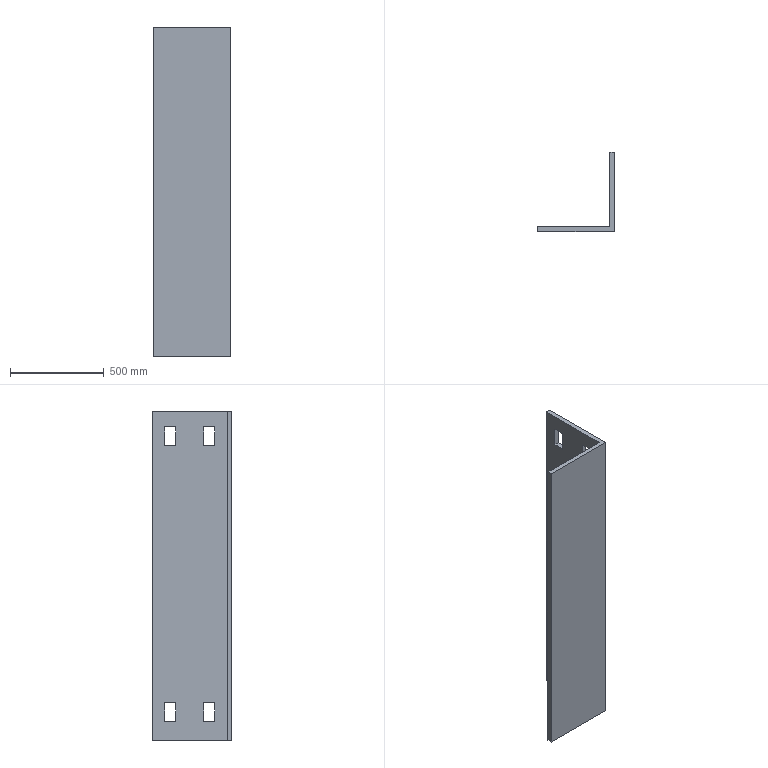Part | SolidWorks | features Extrusion 1, ICE 1 | 1 solid | 24 faces | box 410 x 422.981 x 1750 mm | volume 34749166 mm3 | plane 24
STEP:
#1=CARTESIAN_POINT('',(114.86,92.019,-775.));
#2=VERTEX_POINT('',#1);
#3=CARTESIAN_POINT('',(114.86,152.019,-775.));
#4=VERTEX_POINT('',#3);
#5=CARTESIAN_POINT('',(114.86,152.019,-775.));
#6=DIRECTION('',(0.,1.,0.));
#7=VECTOR('',#6,1000.);
#8=LINE('',#5,#7);
#9=EDGE_CURVE('',#2,#4,#8,.T.);
#10=ORIENTED_EDGE('',*,*,#9,.F.);
#11=CARTESIAN_POINT('',(114.86,92.019,-675.));
#12=VERTEX_POINT('',#11);
#13=CARTESIAN_POINT('',(114.86,92.019,-775.));
#14=DIRECTION('',(0.,0.,-1.));
#15=VECTOR('',#14,1000.);
#16=LINE('',#13,#15);
#17=EDGE_CURVE('',#12,#2,#16,.T.);
#18=ORIENTED_EDGE('',*,*,#17,.F.);
#19=CARTESIAN_POINT('',(114.86,152.019,-675.));
#20=VERTEX_POINT('',#19);
#21=CARTESIAN_POINT('',(114.86,92.019,-675.));
#22=DIRECTION('',(0.,-1.,0.));
#23=VECTOR('',#22,1000.);
#24=LINE('',#21,#23);
#25=EDGE_CURVE('',#20,#12,#24,.T.);
#26=ORIENTED_EDGE('',*,*,#25,.F.);
#27=CARTESIAN_POINT('',(114.86,152.019,-675.));
#28=DIRECTION('',(0.,0.,1.));
#29=VECTOR('',#28,1000.);
#30=LINE('',#27,#29);
#31=EDGE_CURVE('',#4,#20,#30,.T.);
#32=ORIENTED_EDGE('',*,*,#31,.F.);
#33=EDGE_LOOP('',(#10,#18,#26,#32));
#34=FACE_BOUND('',#33,.T.);
#35=CARTESIAN_POINT('',(114.86,360.,-675.));
#36=VERTEX_POINT('',#35);
#37=CARTESIAN_POINT('',(114.86,300.,-675.));
#38=VERTEX_POINT('',#37);
#39=CARTESIAN_POINT('',(114.86,300.,-675.));
#40=DIRECTION('',(0.,-1.,0.));
#41=VECTOR('',#40,1000.);
#42=LINE('',#39,#41);
#43=EDGE_CURVE('',#36,#38,#42,.T.);
#44=ORIENTED_EDGE('',*,*,#43,.F.);
#45=CARTESIAN_POINT('',(114.86,360.,-775.));
#46=VERTEX_POINT('',#45);
#47=CARTESIAN_POINT('',(114.86,360.,-775.));
#48=DIRECTION('',(0.,0.,1.));
#49=VECTOR('',#48,1000.);
#50=LINE('',#47,#49);
#51=EDGE_CURVE('',#46,#36,#50,.T.);
#52=ORIENTED_EDGE('',*,*,#51,.F.);
#53=CARTESIAN_POINT('',(114.86,300.,-775.));
#54=VERTEX_POINT('',#53);
#55=CARTESIAN_POINT('',(114.86,360.,-775.));
#56=DIRECTION('',(0.,1.,0.));
#57=VECTOR('',#56,1000.);
#58=LINE('',#55,#57);
#59=EDGE_CURVE('',#54,#46,#58,.T.);
#60=ORIENTED_EDGE('',*,*,#59,.F.);
#61=CARTESIAN_POINT('',(114.86,300.,-775.));
#62=DIRECTION('',(0.,0.,-1.));
#63=VECTOR('',#62,1000.);
#64=LINE('',#61,#63);
#65=EDGE_CURVE('',#38,#54,#64,.T.);
#66=ORIENTED_EDGE('',*,*,#65,.F.);
#67=EDGE_LOOP('',(#44,#52,#60,#66));
#68=FACE_BOUND('',#67,.T.);
#69=CARTESIAN_POINT('',(114.86,2.019,-875.));
#70=VERTEX_POINT('',#69);
#71=CARTESIAN_POINT('',(114.86,425.,-875.));
#72=VERTEX_POINT('',#71);
#73=CARTESIAN_POINT('',(114.86,2.019,-875.));
#74=DIRECTION('',(0.,1.,0.));
#75=VECTOR('',#74,1000.);
#76=LINE('',#73,#75);
#77=EDGE_CURVE('',#70,#72,#76,.T.);
#78=ORIENTED_EDGE('',*,*,#77,.T.);
#79=CARTESIAN_POINT('',(114.86,425.,875.));
#80=VERTEX_POINT('',#79);
#81=CARTESIAN_POINT('',(114.86,425.,875.));
#82=DIRECTION('',(0.,0.,-1.));
#83=VECTOR('',#82,1000.);
#84=LINE('',#81,#83);
#85=EDGE_CURVE('',#80,#72,#84,.T.);
#86=ORIENTED_EDGE('',*,*,#85,.F.);
#87=CARTESIAN_POINT('',(114.86,2.019,875.));
#88=VERTEX_POINT('',#87);
#89=CARTESIAN_POINT('',(114.86,2.019,875.));
#90=DIRECTION('',(0.,1.,0.));
#91=VECTOR('',#90,1000.);
#92=LINE('',#89,#91);
#93=EDGE_CURVE('',#88,#80,#92,.T.);
#94=ORIENTED_EDGE('',*,*,#93,.F.);
#95=CARTESIAN_POINT('',(114.86,2.019,875.));
#96=DIRECTION('',(0.,0.,-1.));
#97=VECTOR('',#96,1000.);
#98=LINE('',#95,#97);
#99=EDGE_CURVE('',#88,#70,#98,.T.);
#100=ORIENTED_EDGE('',*,*,#99,.T.);
#101=EDGE_LOOP('',(#78,#86,#94,#100));
#102=FACE_OUTER_BOUND('',#101,.T.);
#103=CARTESIAN_POINT('',(114.86,92.019,795.));
#104=VERTEX_POINT('',#103);
#105=CARTESIAN_POINT('',(114.86,92.019,695.));
#106=VERTEX_POINT('',#105);
#107=CARTESIAN_POINT('',(114.86,92.019,695.));
#108=DIRECTION('',(0.,0.,-1.));
#109=VECTOR('',#108,1000.);
#110=LINE('',#107,#109);
#111=EDGE_CURVE('',#104,#106,#110,.T.);
#112=ORIENTED_EDGE('',*,*,#111,.F.);
#113=CARTESIAN_POINT('',(114.86,152.019,795.));
#114=VERTEX_POINT('',#113);
#115=CARTESIAN_POINT('',(114.86,92.019,795.));
#116=DIRECTION('',(0.,-1.,0.));
#117=VECTOR('',#116,1000.);
#118=LINE('',#115,#117);
#119=EDGE_CURVE('',#114,#104,#118,.T.);
#120=ORIENTED_EDGE('',*,*,#119,.F.);
#121=CARTESIAN_POINT('',(114.86,152.019,695.));
#122=VERTEX_POINT('',#121);
#123=CARTESIAN_POINT('',(114.86,152.019,795.));
#124=DIRECTION('',(0.,0.,1.));
#125=VECTOR('',#124,1000.);
#126=LINE('',#123,#125);
#127=EDGE_CURVE('',#122,#114,#126,.T.);
#128=ORIENTED_EDGE('',*,*,#127,.F.);
#129=CARTESIAN_POINT('',(114.86,152.019,695.));
#130=DIRECTION('',(0.,1.,0.));
#131=VECTOR('',#130,1000.);
#132=LINE('',#129,#131);
#133=EDGE_CURVE('',#106,#122,#132,.T.);
#134=ORIENTED_EDGE('',*,*,#133,.F.);
#135=EDGE_LOOP('',(#112,#120,#128,#134));
#136=FACE_BOUND('',#135,.T.);
#137=CARTESIAN_POINT('',(114.86,360.,695.));
#138=VERTEX_POINT('',#137);
#139=CARTESIAN_POINT('',(114.86,360.,795.));
#140=VERTEX_POINT('',#139);
#141=CARTESIAN_POINT('',(114.86,360.,795.));
#142=DIRECTION('',(0.,0.,1.));
#143=VECTOR('',#142,1000.);
#144=LINE('',#141,#143);
#145=EDGE_CURVE('',#138,#140,#144,.T.);
#146=ORIENTED_EDGE('',*,*,#145,.F.);
#147=CARTESIAN_POINT('',(114.86,300.,695.));
#148=VERTEX_POINT('',#147);
#149=CARTESIAN_POINT('',(114.86,360.,695.));
#150=DIRECTION('',(0.,1.,0.));
#151=VECTOR('',#150,1000.);
#152=LINE('',#149,#151);
#153=EDGE_CURVE('',#148,#138,#152,.T.);
#154=ORIENTED_EDGE('',*,*,#153,.F.);
#155=CARTESIAN_POINT('',(114.86,300.,795.));
#156=VERTEX_POINT('',#155);
#157=CARTESIAN_POINT('',(114.86,300.,795.));
#158=DIRECTION('',(0.,0.,-1.));
#159=VECTOR('',#158,1000.);
#160=LINE('',#157,#159);
#161=EDGE_CURVE('',#156,#148,#160,.T.);
#162=ORIENTED_EDGE('',*,*,#161,.F.);
#163=CARTESIAN_POINT('',(114.86,300.,795.));
#164=DIRECTION('',(0.,-1.,0.));
#165=VECTOR('',#164,1000.);
#166=LINE('',#163,#165);
#167=EDGE_CURVE('',#140,#156,#166,.T.);
#168=ORIENTED_EDGE('',*,*,#167,.F.);
#169=EDGE_LOOP('',(#146,#154,#162,#168));
#170=FACE_BOUND('',#169,.T.);
#171=CARTESIAN_POINT('',(114.86,2.019,875.));
#172=DIRECTION('',(-1.,0.,0.));
#173=DIRECTION('',(0.,0.,1.));
#174=AXIS2_PLACEMENT_3D('',#171,#172,#173);
#175=PLANE('',#174);
#176=ADVANCED_FACE('',(#34,#68,#102,#136,#170),#175,.F.);
#177=CARTESIAN_POINT('',(89.86,152.019,-775.));
#178=VERTEX_POINT('',#177);
#179=CARTESIAN_POINT('',(89.86,92.019,-775.));
#180=VERTEX_POINT('',#179);
#181=CARTESIAN_POINT('',(89.86,425.,-775.));
#182=DIRECTION('',(0.,-1.,0.));
#183=VECTOR('',#182,1000.);
#184=LINE('',#181,#183);
#185=EDGE_CURVE('',#178,#180,#184,.T.);
#186=ORIENTED_EDGE('',*,*,#185,.F.);
#187=CARTESIAN_POINT('',(89.86,152.019,-675.));
#188=VERTEX_POINT('',#187);
#189=CARTESIAN_POINT('',(89.86,152.019,875.));
#190=DIRECTION('',(0.,0.,-1.));
#191=VECTOR('',#190,1000.);
#192=LINE('',#189,#191);
#193=EDGE_CURVE('',#188,#178,#192,.T.);
#194=ORIENTED_EDGE('',*,*,#193,.F.);
#195=CARTESIAN_POINT('',(89.86,92.019,-675.));
#196=VERTEX_POINT('',#195);
#197=CARTESIAN_POINT('',(89.86,425.,-675.));
#198=DIRECTION('',(0.,1.,0.));
#199=VECTOR('',#198,1000.);
#200=LINE('',#197,#199);
#201=EDGE_CURVE('',#196,#188,#200,.T.);
#202=ORIENTED_EDGE('',*,*,#201,.F.);
#203=CARTESIAN_POINT('',(89.86,92.019,875.));
#204=DIRECTION('',(0.,0.,1.));
#205=VECTOR('',#204,1000.);
#206=LINE('',#203,#205);
#207=EDGE_CURVE('',#180,#196,#206,.T.);
#208=ORIENTED_EDGE('',*,*,#207,.F.);
#209=EDGE_LOOP('',(#186,#194,#202,#208));
#210=FACE_BOUND('',#209,.T.);
#211=CARTESIAN_POINT('',(89.86,300.,-675.));
#212=VERTEX_POINT('',#211);
#213=CARTESIAN_POINT('',(89.86,360.,-675.));
#214=VERTEX_POINT('',#213);
#215=CARTESIAN_POINT('',(89.86,425.,-675.));
#216=DIRECTION('',(0.,1.,0.));
#217=VECTOR('',#216,1000.);
#218=LINE('',#215,#217);
#219=EDGE_CURVE('',#212,#214,#218,.T.);
#220=ORIENTED_EDGE('',*,*,#219,.F.);
#221=CARTESIAN_POINT('',(89.86,300.,-775.));
#222=VERTEX_POINT('',#221);
#223=CARTESIAN_POINT('',(89.86,300.,875.));
#224=DIRECTION('',(0.,0.,1.));
#225=VECTOR('',#224,1000.);
#226=LINE('',#223,#225);
#227=EDGE_CURVE('',#222,#212,#226,.T.);
#228=ORIENTED_EDGE('',*,*,#227,.F.);
#229=CARTESIAN_POINT('',(89.86,360.,-775.));
#230=VERTEX_POINT('',#229);
#231=CARTESIAN_POINT('',(89.86,425.,-775.));
#232=DIRECTION('',(0.,-1.,0.));
#233=VECTOR('',#232,1000.);
#234=LINE('',#231,#233);
#235=EDGE_CURVE('',#230,#222,#234,.T.);
#236=ORIENTED_EDGE('',*,*,#235,.F.);
#237=CARTESIAN_POINT('',(89.86,360.,875.));
#238=DIRECTION('',(0.,0.,-1.));
#239=VECTOR('',#238,1000.);
#240=LINE('',#237,#239);
#241=EDGE_CURVE('',#214,#230,#240,.T.);
#242=ORIENTED_EDGE('',*,*,#241,.F.);
#243=EDGE_LOOP('',(#220,#228,#236,#242));
#244=FACE_BOUND('',#243,.T.);
#245=CARTESIAN_POINT('',(89.86,425.,-875.));
#246=VERTEX_POINT('',#245);
#247=CARTESIAN_POINT('',(89.86,27.019,-875.));
#248=VERTEX_POINT('',#247);
#249=CARTESIAN_POINT('',(89.86,425.,-875.));
#250=DIRECTION('',(0.,-1.,0.));
#251=VECTOR('',#250,1000.);
#252=LINE('',#249,#251);
#253=EDGE_CURVE('',#246,#248,#252,.T.);
#254=ORIENTED_EDGE('',*,*,#253,.T.);
#255=CARTESIAN_POINT('',(89.86,27.019,875.));
#256=VERTEX_POINT('',#255);
#257=CARTESIAN_POINT('',(89.86,27.019,875.));
#258=DIRECTION('',(0.,0.,-1.));
#259=VECTOR('',#258,1000.);
#260=LINE('',#257,#259);
#261=EDGE_CURVE('',#256,#248,#260,.T.);
#262=ORIENTED_EDGE('',*,*,#261,.F.);
#263=CARTESIAN_POINT('',(89.86,425.,875.));
#264=VERTEX_POINT('',#263);
#265=CARTESIAN_POINT('',(89.86,425.,875.));
#266=DIRECTION('',(0.,-1.,0.));
#267=VECTOR('',#266,1000.);
#268=LINE('',#265,#267);
#269=EDGE_CURVE('',#264,#256,#268,.T.);
#270=ORIENTED_EDGE('',*,*,#269,.F.);
#271=CARTESIAN_POINT('',(89.86,425.,875.));
#272=DIRECTION('',(0.,0.,-1.));
#273=VECTOR('',#272,1000.);
#274=LINE('',#271,#273);
#275=EDGE_CURVE('',#264,#246,#274,.T.);
#276=ORIENTED_EDGE('',*,*,#275,.T.);
#277=EDGE_LOOP('',(#254,#262,#270,#276));
#278=FACE_OUTER_BOUND('',#277,.T.);
#279=CARTESIAN_POINT('',(89.86,92.019,695.));
#280=VERTEX_POINT('',#279);
#281=CARTESIAN_POINT('',(89.86,92.019,795.));
#282=VERTEX_POINT('',#281);
#283=CARTESIAN_POINT('',(89.86,92.019,875.));
#284=DIRECTION('',(0.,0.,1.));
#285=VECTOR('',#284,1000.);
#286=LINE('',#283,#285);
#287=EDGE_CURVE('',#280,#282,#286,.T.);
#288=ORIENTED_EDGE('',*,*,#287,.F.);
#289=CARTESIAN_POINT('',(89.86,152.019,695.));
#290=VERTEX_POINT('',#289);
#291=CARTESIAN_POINT('',(89.86,425.,695.));
#292=DIRECTION('',(0.,-1.,0.));
#293=VECTOR('',#292,1000.);
#294=LINE('',#291,#293);
#295=EDGE_CURVE('',#290,#280,#294,.T.);
#296=ORIENTED_EDGE('',*,*,#295,.F.);
#297=CARTESIAN_POINT('',(89.86,152.019,795.));
#298=VERTEX_POINT('',#297);
#299=CARTESIAN_POINT('',(89.86,152.019,875.));
#300=DIRECTION('',(0.,0.,-1.));
#301=VECTOR('',#300,1000.);
#302=LINE('',#299,#301);
#303=EDGE_CURVE('',#298,#290,#302,.T.);
#304=ORIENTED_EDGE('',*,*,#303,.F.);
#305=CARTESIAN_POINT('',(89.86,425.,795.));
#306=DIRECTION('',(0.,1.,0.));
#307=VECTOR('',#306,1000.);
#308=LINE('',#305,#307);
#309=EDGE_CURVE('',#282,#298,#308,.T.);
#310=ORIENTED_EDGE('',*,*,#309,.F.);
#311=EDGE_LOOP('',(#288,#296,#304,#310));
#312=FACE_BOUND('',#311,.T.);
#313=CARTESIAN_POINT('',(89.86,360.,795.));
#314=VERTEX_POINT('',#313);
#315=CARTESIAN_POINT('',(89.86,360.,695.));
#316=VERTEX_POINT('',#315);
#317=CARTESIAN_POINT('',(89.86,360.,875.));
#318=DIRECTION('',(0.,0.,-1.));
#319=VECTOR('',#318,1000.);
#320=LINE('',#317,#319);
#321=EDGE_CURVE('',#314,#316,#320,.T.);
#322=ORIENTED_EDGE('',*,*,#321,.F.);
#323=CARTESIAN_POINT('',(89.86,300.,795.));
#324=VERTEX_POINT('',#323);
#325=CARTESIAN_POINT('',(89.86,425.,795.));
#326=DIRECTION('',(0.,1.,0.));
#327=VECTOR('',#326,1000.);
#328=LINE('',#325,#327);
#329=EDGE_CURVE('',#324,#314,#328,.T.);
#330=ORIENTED_EDGE('',*,*,#329,.F.);
#331=CARTESIAN_POINT('',(89.86,300.,695.));
#332=VERTEX_POINT('',#331);
#333=CARTESIAN_POINT('',(89.86,300.,875.));
#334=DIRECTION('',(0.,0.,1.));
#335=VECTOR('',#334,1000.);
#336=LINE('',#333,#335);
#337=EDGE_CURVE('',#332,#324,#336,.T.);
#338=ORIENTED_EDGE('',*,*,#337,.F.);
#339=CARTESIAN_POINT('',(89.86,425.,695.));
#340=DIRECTION('',(0.,-1.,0.));
#341=VECTOR('',#340,1000.);
#342=LINE('',#339,#341);
#343=EDGE_CURVE('',#316,#332,#342,.T.);
#344=ORIENTED_EDGE('',*,*,#343,.F.);
#345=EDGE_LOOP('',(#322,#330,#338,#344));
#346=FACE_BOUND('',#345,.T.);
#347=CARTESIAN_POINT('',(89.86,425.,875.));
#348=DIRECTION('',(1.,0.,0.));
#349=DIRECTION('',(0.,0.,-1.));
#350=AXIS2_PLACEMENT_3D('',#347,#348,#349);
#351=PLANE('',#350);
#352=ADVANCED_FACE('',(#210,#244,#278,#312,#346),#351,.F.);
#353=CARTESIAN_POINT('',(-295.14,2.019,-875.));
#354=VERTEX_POINT('',#353);
#355=CARTESIAN_POINT('',(-295.14,2.019,-875.));
#356=DIRECTION('',(1.,0.,0.));
#357=VECTOR('',#356,1000.);
#358=LINE('',#355,#357);
#359=EDGE_CURVE('',#354,#70,#358,.T.);
#360=ORIENTED_EDGE('',*,*,#359,.T.);
#361=ORIENTED_EDGE('',*,*,#99,.F.);
#362=CARTESIAN_POINT('',(-295.14,2.019,875.));
#363=VERTEX_POINT('',#362);
#364=CARTESIAN_POINT('',(-295.14,2.019,875.));
#365=DIRECTION('',(1.,0.,0.));
#366=VECTOR('',#365,1000.);
#367=LINE('',#364,#366);
#368=EDGE_CURVE('',#363,#88,#367,.T.);
#369=ORIENTED_EDGE('',*,*,#368,.F.);
#370=CARTESIAN_POINT('',(-295.14,2.019,875.));
#371=DIRECTION('',(0.,0.,-1.));
#372=VECTOR('',#371,1000.);
#373=LINE('',#370,#372);
#374=EDGE_CURVE('',#363,#354,#373,.T.);
#375=ORIENTED_EDGE('',*,*,#374,.T.);
#376=EDGE_LOOP('',(#360,#361,#369,#375));
#377=FACE_OUTER_BOUND('',#376,.T.);
#378=CARTESIAN_POINT('',(-295.14,2.019,875.));
#379=DIRECTION('',(0.,1.,0.));
#380=DIRECTION('',(0.,0.,1.));
#381=AXIS2_PLACEMENT_3D('',#378,#379,#380);
#382=PLANE('',#381);
#383=ADVANCED_FACE('',(#377),#382,.F.);
#384=CARTESIAN_POINT('',(114.86,425.,-875.));
#385=DIRECTION('',(-1.,0.,0.));
#386=VECTOR('',#385,1000.);
#387=LINE('',#384,#386);
#388=EDGE_CURVE('',#72,#246,#387,.T.);
#389=ORIENTED_EDGE('',*,*,#388,.T.);
#390=ORIENTED_EDGE('',*,*,#275,.F.);
#391=CARTESIAN_POINT('',(114.86,425.,875.));
#392=DIRECTION('',(-1.,0.,0.));
#393=VECTOR('',#392,1000.);
#394=LINE('',#391,#393);
#395=EDGE_CURVE('',#80,#264,#394,.T.);
#396=ORIENTED_EDGE('',*,*,#395,.F.);
#397=ORIENTED_EDGE('',*,*,#85,.T.);
#398=EDGE_LOOP('',(#389,#390,#396,#397));
#399=FACE_OUTER_BOUND('',#398,.T.);
#400=CARTESIAN_POINT('',(114.86,425.,875.));
#401=DIRECTION('',(0.,-1.,0.));
#402=DIRECTION('',(0.,0.,-1.));
#403=AXIS2_PLACEMENT_3D('',#400,#401,#402);
#404=PLANE('',#403);
#405=ADVANCED_FACE('',(#399),#404,.F.);
#406=CARTESIAN_POINT('',(-295.14,27.019,-875.));
#407=VERTEX_POINT('',#406);
#408=CARTESIAN_POINT('',(89.86,27.019,-875.));
#409=DIRECTION('',(-1.,0.,0.));
#410=VECTOR('',#409,1000.);
#411=LINE('',#408,#410);
#412=EDGE_CURVE('',#248,#407,#411,.T.);
#413=ORIENTED_EDGE('',*,*,#412,.T.);
#414=CARTESIAN_POINT('',(-295.14,27.019,875.));
#415=VERTEX_POINT('',#414);
#416=CARTESIAN_POINT('',(-295.14,27.019,875.));
#417=DIRECTION('',(0.,0.,-1.));
#418=VECTOR('',#417,1000.);
#419=LINE('',#416,#418);
#420=EDGE_CURVE('',#415,#407,#419,.T.);
#421=ORIENTED_EDGE('',*,*,#420,.F.);
#422=CARTESIAN_POINT('',(89.86,27.019,875.));
#423=DIRECTION('',(-1.,0.,0.));
#424=VECTOR('',#423,1000.);
#425=LINE('',#422,#424);
#426=EDGE_CURVE('',#256,#415,#425,.T.);
#427=ORIENTED_EDGE('',*,*,#426,.F.);
#428=ORIENTED_EDGE('',*,*,#261,.T.);
#429=EDGE_LOOP('',(#413,#421,#427,#428));
#430=FACE_OUTER_BOUND('',#429,.T.);
#431=CARTESIAN_POINT('',(89.86,27.019,875.));
#432=DIRECTION('',(0.,-1.,0.));
#433=DIRECTION('',(1.,0.,0.));
#434=AXIS2_PLACEMENT_3D('',#431,#432,#433);
#435=PLANE('',#434);
#436=ADVANCED_FACE('',(#430),#435,.F.);
#437=CARTESIAN_POINT('',(-295.14,27.019,-875.));
#438=DIRECTION('',(0.,-1.,0.));
#439=VECTOR('',#438,1000.);
#440=LINE('',#437,#439);
#441=EDGE_CURVE('',#407,#354,#440,.T.);
#442=ORIENTED_EDGE('',*,*,#441,.T.);
#443=ORIENTED_EDGE('',*,*,#374,.F.);
#444=CARTESIAN_POINT('',(-295.14,27.019,875.));
#445=DIRECTION('',(0.,-1.,0.));
#446=VECTOR('',#445,1000.);
#447=LINE('',#444,#446);
#448=EDGE_CURVE('',#415,#363,#447,.T.);
#449=ORIENTED_EDGE('',*,*,#448,.F.);
#450=ORIENTED_EDGE('',*,*,#420,.T.);
#451=EDGE_LOOP('',(#442,#443,#449,#450));
#452=FACE_OUTER_BOUND('',#451,.T.);
#453=CARTESIAN_POINT('',(-295.14,27.019,875.));
#454=DIRECTION('',(1.,0.,0.));
#455=DIRECTION('',(0.,0.,-1.));
#456=AXIS2_PLACEMENT_3D('',#453,#454,#455);
#457=PLANE('',#456);
#458=ADVANCED_FACE('',(#452),#457,.F.);
#459=ORIENTED_EDGE('',*,*,#368,.T.);
#460=ORIENTED_EDGE('',*,*,#93,.T.);
#461=ORIENTED_EDGE('',*,*,#395,.T.);
#462=ORIENTED_EDGE('',*,*,#269,.T.);
#463=ORIENTED_EDGE('',*,*,#426,.T.);
#464=ORIENTED_EDGE('',*,*,#448,.T.);
#465=EDGE_LOOP('',(#459,#460,#461,#462,#463,#464));
#466=FACE_OUTER_BOUND('',#465,.T.);
#467=CARTESIAN_POINT('',(0.,0.,875.));
#468=DIRECTION('',(0.,0.,1.));
#469=DIRECTION('',(1.,0.,0.));
#470=AXIS2_PLACEMENT_3D('',#467,#468,#469);
#471=PLANE('',#470);
#472=ADVANCED_FACE('',(#466),#471,.T.);
#473=ORIENTED_EDGE('',*,*,#359,.F.);
#474=ORIENTED_EDGE('',*,*,#441,.F.);
#475=ORIENTED_EDGE('',*,*,#412,.F.);
#476=ORIENTED_EDGE('',*,*,#253,.F.);
#477=ORIENTED_EDGE('',*,*,#388,.F.);
#478=ORIENTED_EDGE('',*,*,#77,.F.);
#479=EDGE_LOOP('',(#473,#474,#475,#476,#477,#478));
#480=FACE_OUTER_BOUND('',#479,.T.);
#481=CARTESIAN_POINT('',(0.,0.,-875.));
#482=DIRECTION('',(0.,0.,1.));
#483=DIRECTION('',(1.,0.,0.));
#484=AXIS2_PLACEMENT_3D('',#481,#482,#483);
#485=PLANE('',#484);
#486=ADVANCED_FACE('',(#480),#485,.F.);
#487=ORIENTED_EDGE('',*,*,#219,.T.);
#488=CARTESIAN_POINT('',(114.86,360.,-675.));
#489=DIRECTION('',(-1.,0.,0.));
#490=VECTOR('',#489,1000.);
#491=LINE('',#488,#490);
#492=EDGE_CURVE('',#36,#214,#491,.T.);
#493=ORIENTED_EDGE('',*,*,#492,.F.);
#494=ORIENTED_EDGE('',*,*,#43,.T.);
#495=CARTESIAN_POINT('',(114.86,300.,-675.));
#496=DIRECTION('',(-1.,0.,0.));
#497=VECTOR('',#496,1000.);
#498=LINE('',#495,#497);
#499=EDGE_CURVE('',#38,#212,#498,.T.);
#500=ORIENTED_EDGE('',*,*,#499,.T.);
#501=EDGE_LOOP('',(#487,#493,#494,#500));
#502=FACE_OUTER_BOUND('',#501,.T.);
#503=CARTESIAN_POINT('',(114.86,300.,-675.));
#504=DIRECTION('',(0.,0.,-1.));
#505=DIRECTION('',(-1.,0.,0.));
#506=AXIS2_PLACEMENT_3D('',#503,#504,#505);
#507=PLANE('',#506);
#508=ADVANCED_FACE('',(#502),#507,.T.);
#509=ORIENTED_EDGE('',*,*,#227,.T.);
#510=ORIENTED_EDGE('',*,*,#499,.F.);
#511=ORIENTED_EDGE('',*,*,#65,.T.);
#512=CARTESIAN_POINT('',(114.86,300.,-775.));
#513=DIRECTION('',(-1.,0.,0.));
#514=VECTOR('',#513,1000.);
#515=LINE('',#512,#514);
#516=EDGE_CURVE('',#54,#222,#515,.T.);
#517=ORIENTED_EDGE('',*,*,#516,.T.);
#518=EDGE_LOOP('',(#509,#510,#511,#517));
#519=FACE_OUTER_BOUND('',#518,.T.);
#520=CARTESIAN_POINT('',(114.86,300.,-775.));
#521=DIRECTION('',(0.,1.,0.));
#522=DIRECTION('',(0.,0.,1.));
#523=AXIS2_PLACEMENT_3D('',#520,#521,#522);
#524=PLANE('',#523);
#525=ADVANCED_FACE('',(#519),#524,.T.);
#526=ORIENTED_EDGE('',*,*,#235,.T.);
#527=ORIENTED_EDGE('',*,*,#516,.F.);
#528=ORIENTED_EDGE('',*,*,#59,.T.);
#529=CARTESIAN_POINT('',(114.86,360.,-775.));
#530=DIRECTION('',(-1.,0.,0.));
#531=VECTOR('',#530,1000.);
#532=LINE('',#529,#531);
#533=EDGE_CURVE('',#46,#230,#532,.T.);
#534=ORIENTED_EDGE('',*,*,#533,.T.);
#535=EDGE_LOOP('',(#526,#527,#528,#534));
#536=FACE_OUTER_BOUND('',#535,.T.);
#537=CARTESIAN_POINT('',(114.86,360.,-775.));
#538=DIRECTION('',(0.,0.,1.));
#539=DIRECTION('',(1.,0.,0.));
#540=AXIS2_PLACEMENT_3D('',#537,#538,#539);
#541=PLANE('',#540);
#542=ADVANCED_FACE('',(#536),#541,.T.);
#543=ORIENTED_EDGE('',*,*,#241,.T.);
#544=ORIENTED_EDGE('',*,*,#533,.F.);
#545=ORIENTED_EDGE('',*,*,#51,.T.);
#546=ORIENTED_EDGE('',*,*,#492,.T.);
#547=EDGE_LOOP('',(#543,#544,#545,#546));
#548=FACE_OUTER_BOUND('',#547,.T.);
#549=CARTESIAN_POINT('',(114.86,360.,-775.));
#550=DIRECTION('',(0.,-1.,0.));
#551=DIRECTION('',(0.,0.,-1.));
#552=AXIS2_PLACEMENT_3D('',#549,#550,#551);
#553=PLANE('',#552);
#554=ADVANCED_FACE('',(#548),#553,.T.);
#555=ORIENTED_EDGE('',*,*,#287,.T.);
#556=CARTESIAN_POINT('',(114.86,92.019,795.));
#557=DIRECTION('',(-1.,0.,0.));
#558=VECTOR('',#557,1000.);
#559=LINE('',#556,#558);
#560=EDGE_CURVE('',#104,#282,#559,.T.);
#561=ORIENTED_EDGE('',*,*,#560,.F.);
#562=ORIENTED_EDGE('',*,*,#111,.T.);
#563=CARTESIAN_POINT('',(114.86,92.019,695.));
#564=DIRECTION('',(-1.,0.,0.));
#565=VECTOR('',#564,1000.);
#566=LINE('',#563,#565);
#567=EDGE_CURVE('',#106,#280,#566,.T.);
#568=ORIENTED_EDGE('',*,*,#567,.T.);
#569=EDGE_LOOP('',(#555,#561,#562,#568));
#570=FACE_OUTER_BOUND('',#569,.T.);
#571=CARTESIAN_POINT('',(114.86,92.019,695.));
#572=DIRECTION('',(0.,1.,0.));
#573=DIRECTION('',(0.,0.,1.));
#574=AXIS2_PLACEMENT_3D('',#571,#572,#573);
#575=PLANE('',#574);
#576=ADVANCED_FACE('',(#570),#575,.T.);
#577=ORIENTED_EDGE('',*,*,#295,.T.);
#578=ORIENTED_EDGE('',*,*,#567,.F.);
#579=ORIENTED_EDGE('',*,*,#133,.T.);
#580=CARTESIAN_POINT('',(114.86,152.019,695.));
#581=DIRECTION('',(-1.,0.,0.));
#582=VECTOR('',#581,1000.);
#583=LINE('',#580,#582);
#584=EDGE_CURVE('',#122,#290,#583,.T.);
#585=ORIENTED_EDGE('',*,*,#584,.T.);
#586=EDGE_LOOP('',(#577,#578,#579,#585));
#587=FACE_OUTER_BOUND('',#586,.T.);
#588=CARTESIAN_POINT('',(114.86,152.019,695.));
#589=DIRECTION('',(0.,0.,1.));
#590=DIRECTION('',(1.,0.,0.));
#591=AXIS2_PLACEMENT_3D('',#588,#589,#590);
#592=PLANE('',#591);
#593=ADVANCED_FACE('',(#587),#592,.T.);
#594=ORIENTED_EDGE('',*,*,#303,.T.);
#595=ORIENTED_EDGE('',*,*,#584,.F.);
#596=ORIENTED_EDGE('',*,*,#127,.T.);
#597=CARTESIAN_POINT('',(114.86,152.019,795.));
#598=DIRECTION('',(-1.,0.,0.));
#599=VECTOR('',#598,1000.);
#600=LINE('',#597,#599);
#601=EDGE_CURVE('',#114,#298,#600,.T.);
#602=ORIENTED_EDGE('',*,*,#601,.T.);
#603=EDGE_LOOP('',(#594,#595,#596,#602));
#604=FACE_OUTER_BOUND('',#603,.T.);
#605=CARTESIAN_POINT('',(114.86,152.019,795.));
#606=DIRECTION('',(0.,-1.,0.));
#607=DIRECTION('',(0.,0.,-1.));
#608=AXIS2_PLACEMENT_3D('',#605,#606,#607);
#609=PLANE('',#608);
#610=ADVANCED_FACE('',(#604),#609,.T.);
#611=ORIENTED_EDGE('',*,*,#309,.T.);
#612=ORIENTED_EDGE('',*,*,#601,.F.);
#613=ORIENTED_EDGE('',*,*,#119,.T.);
#614=ORIENTED_EDGE('',*,*,#560,.T.);
#615=EDGE_LOOP('',(#611,#612,#613,#614));
#616=FACE_OUTER_BOUND('',#615,.T.);
#617=CARTESIAN_POINT('',(114.86,92.019,795.));
#618=DIRECTION('',(0.,0.,-1.));
#619=DIRECTION('',(-1.,0.,0.));
#620=AXIS2_PLACEMENT_3D('',#617,#618,#619);
#621=PLANE('',#620);
#622=ADVANCED_FACE('',(#616),#621,.T.);
#623=ORIENTED_EDGE('',*,*,#185,.T.);
#624=CARTESIAN_POINT('',(114.86,92.019,-775.));
#625=DIRECTION('',(-1.,0.,0.));
#626=VECTOR('',#625,1000.);
#627=LINE('',#624,#626);
#628=EDGE_CURVE('',#2,#180,#627,.T.);
#629=ORIENTED_EDGE('',*,*,#628,.F.);
#630=ORIENTED_EDGE('',*,*,#9,.T.);
#631=CARTESIAN_POINT('',(114.86,152.019,-775.));
#632=DIRECTION('',(-1.,0.,0.));
#633=VECTOR('',#632,1000.);
#634=LINE('',#631,#633);
#635=EDGE_CURVE('',#4,#178,#634,.T.);
#636=ORIENTED_EDGE('',*,*,#635,.T.);
#637=EDGE_LOOP('',(#623,#629,#630,#636));
#638=FACE_OUTER_BOUND('',#637,.T.);
#639=CARTESIAN_POINT('',(114.86,152.019,-775.));
#640=DIRECTION('',(0.,0.,1.));
#641=DIRECTION('',(1.,0.,0.));
#642=AXIS2_PLACEMENT_3D('',#639,#640,#641);
#643=PLANE('',#642);
#644=ADVANCED_FACE('',(#638),#643,.T.);
#645=ORIENTED_EDGE('',*,*,#193,.T.);
#646=ORIENTED_EDGE('',*,*,#635,.F.);
#647=ORIENTED_EDGE('',*,*,#31,.T.);
#648=CARTESIAN_POINT('',(114.86,152.019,-675.));
#649=DIRECTION('',(-1.,0.,0.));
#650=VECTOR('',#649,1000.);
#651=LINE('',#648,#650);
#652=EDGE_CURVE('',#20,#188,#651,.T.);
#653=ORIENTED_EDGE('',*,*,#652,.T.);
#654=EDGE_LOOP('',(#645,#646,#647,#653));
#655=FACE_OUTER_BOUND('',#654,.T.);
#656=CARTESIAN_POINT('',(114.86,152.019,-675.));
#657=DIRECTION('',(0.,-1.,0.));
#658=DIRECTION('',(0.,0.,-1.));
#659=AXIS2_PLACEMENT_3D('',#656,#657,#658);
#660=PLANE('',#659);
#661=ADVANCED_FACE('',(#655),#660,.T.);
#662=ORIENTED_EDGE('',*,*,#201,.T.);
#663=ORIENTED_EDGE('',*,*,#652,.F.);
#664=ORIENTED_EDGE('',*,*,#25,.T.);
#665=CARTESIAN_POINT('',(114.86,92.019,-675.));
#666=DIRECTION('',(-1.,0.,0.));
#667=VECTOR('',#666,1000.);
#668=LINE('',#665,#667);
#669=EDGE_CURVE('',#12,#196,#668,.T.);
#670=ORIENTED_EDGE('',*,*,#669,.T.);
#671=EDGE_LOOP('',(#662,#663,#664,#670));
#672=FACE_OUTER_BOUND('',#671,.T.);
#673=CARTESIAN_POINT('',(114.86,92.019,-675.));
#674=DIRECTION('',(0.,0.,-1.));
#675=DIRECTION('',(-1.,0.,0.));
#676=AXIS2_PLACEMENT_3D('',#673,#674,#675);
#677=PLANE('',#676);
#678=ADVANCED_FACE('',(#672),#677,.T.);
#679=ORIENTED_EDGE('',*,*,#207,.T.);
#680=ORIENTED_EDGE('',*,*,#669,.F.);
#681=ORIENTED_EDGE('',*,*,#17,.T.);
#682=ORIENTED_EDGE('',*,*,#628,.T.);
#683=EDGE_LOOP('',(#679,#680,#681,#682));
#684=FACE_OUTER_BOUND('',#683,.T.);
#685=CARTESIAN_POINT('',(114.86,92.019,-775.));
#686=DIRECTION('',(0.,1.,0.));
#687=DIRECTION('',(0.,0.,1.));
#688=AXIS2_PLACEMENT_3D('',#685,#686,#687);
#689=PLANE('',#688);
#690=ADVANCED_FACE('',(#684),#689,.T.);
#691=ORIENTED_EDGE('',*,*,#321,.T.);
#692=CARTESIAN_POINT('',(114.86,360.,695.));
#693=DIRECTION('',(-1.,0.,0.));
#694=VECTOR('',#693,1000.);
#695=LINE('',#692,#694);
#696=EDGE_CURVE('',#138,#316,#695,.T.);
#697=ORIENTED_EDGE('',*,*,#696,.F.);
#698=ORIENTED_EDGE('',*,*,#145,.T.);
#699=CARTESIAN_POINT('',(114.86,360.,795.));
#700=DIRECTION('',(-1.,0.,0.));
#701=VECTOR('',#700,1000.);
#702=LINE('',#699,#701);
#703=EDGE_CURVE('',#140,#314,#702,.T.);
#704=ORIENTED_EDGE('',*,*,#703,.T.);
#705=EDGE_LOOP('',(#691,#697,#698,#704));
#706=FACE_OUTER_BOUND('',#705,.T.);
#707=CARTESIAN_POINT('',(114.86,360.,795.));
#708=DIRECTION('',(0.,-1.,0.));
#709=DIRECTION('',(0.,0.,-1.));
#710=AXIS2_PLACEMENT_3D('',#707,#708,#709);
#711=PLANE('',#710);
#712=ADVANCED_FACE('',(#706),#711,.T.);
#713=ORIENTED_EDGE('',*,*,#329,.T.);
#714=ORIENTED_EDGE('',*,*,#703,.F.);
#715=ORIENTED_EDGE('',*,*,#167,.T.);
#716=CARTESIAN_POINT('',(114.86,300.,795.));
#717=DIRECTION('',(-1.,0.,0.));
#718=VECTOR('',#717,1000.);
#719=LINE('',#716,#718);
#720=EDGE_CURVE('',#156,#324,#719,.T.);
#721=ORIENTED_EDGE('',*,*,#720,.T.);
#722=EDGE_LOOP('',(#713,#714,#715,#721));
#723=FACE_OUTER_BOUND('',#722,.T.);
#724=CARTESIAN_POINT('',(114.86,300.,795.));
#725=DIRECTION('',(0.,0.,-1.));
#726=DIRECTION('',(-1.,0.,0.));
#727=AXIS2_PLACEMENT_3D('',#724,#725,#726);
#728=PLANE('',#727);
#729=ADVANCED_FACE('',(#723),#728,.T.);
#730=ORIENTED_EDGE('',*,*,#337,.T.);
#731=ORIENTED_EDGE('',*,*,#720,.F.);
#732=ORIENTED_EDGE('',*,*,#161,.T.);
#733=CARTESIAN_POINT('',(114.86,300.,695.));
#734=DIRECTION('',(-1.,0.,0.));
#735=VECTOR('',#734,1000.);
#736=LINE('',#733,#735);
#737=EDGE_CURVE('',#148,#332,#736,.T.);
#738=ORIENTED_EDGE('',*,*,#737,.T.);
#739=EDGE_LOOP('',(#730,#731,#732,#738));
#740=FACE_OUTER_BOUND('',#739,.T.);
#741=CARTESIAN_POINT('',(114.86,300.,795.));
#742=DIRECTION('',(0.,1.,0.));
#743=DIRECTION('',(0.,0.,1.));
#744=AXIS2_PLACEMENT_3D('',#741,#742,#743);
#745=PLANE('',#744);
#746=ADVANCED_FACE('',(#740),#745,.T.);
#747=ORIENTED_EDGE('',*,*,#343,.T.);
#748=ORIENTED_EDGE('',*,*,#737,.F.);
#749=ORIENTED_EDGE('',*,*,#153,.T.);
#750=ORIENTED_EDGE('',*,*,#696,.T.);
#751=EDGE_LOOP('',(#747,#748,#749,#750));
#752=FACE_OUTER_BOUND('',#751,.T.);
#753=CARTESIAN_POINT('',(114.86,360.,695.));
#754=DIRECTION('',(0.,0.,1.));
#755=DIRECTION('',(1.,0.,0.));
#756=AXIS2_PLACEMENT_3D('',#753,#754,#755);
#757=PLANE('',#756);
#758=ADVANCED_FACE('',(#752),#757,.T.);
#759=CLOSED_SHELL('',(#176,#352,#383,#405,#436,#458,#472,#486,#508,#525,#542,#554,#576,#593,#610,#622,#644,#661,#678,#690,#712,#729,#746,#758));
#760=MANIFOLD_SOLID_BREP('',#759);
#761=CARTESIAN_POINT('',(0.,0.,0.));
#762=DIRECTION('',(0.,0.,1.));
#763=DIRECTION('',(1.,0.,0.));
#764=AXIS2_PLACEMENT_3D('',#761,#762,#763);
#765=(LENGTH_UNIT()NAMED_UNIT(*)SI_UNIT(.MILLI.,.METRE.));
#766=UNCERTAINTY_MEASURE_WITH_UNIT(LENGTH_MEASURE(0.00001),#765,'','');
#767=(NAMED_UNIT(*)PLANE_ANGLE_UNIT()SI_UNIT($,.RADIAN.));
#768=(NAMED_UNIT(*)SI_UNIT($,.STERADIAN.)SOLID_ANGLE_UNIT());
#769=(GEOMETRIC_REPRESENTATION_CONTEXT(3)GLOBAL_UNCERTAINTY_ASSIGNED_CONTEXT((#766))GLOBAL_UNIT_ASSIGNED_CONTEXT((#765,#767,#768))REPRESENTATION_CONTEXT('',''));
#770=ADVANCED_BREP_SHAPE_REPRESENTATION('',(#760,#764),#769);